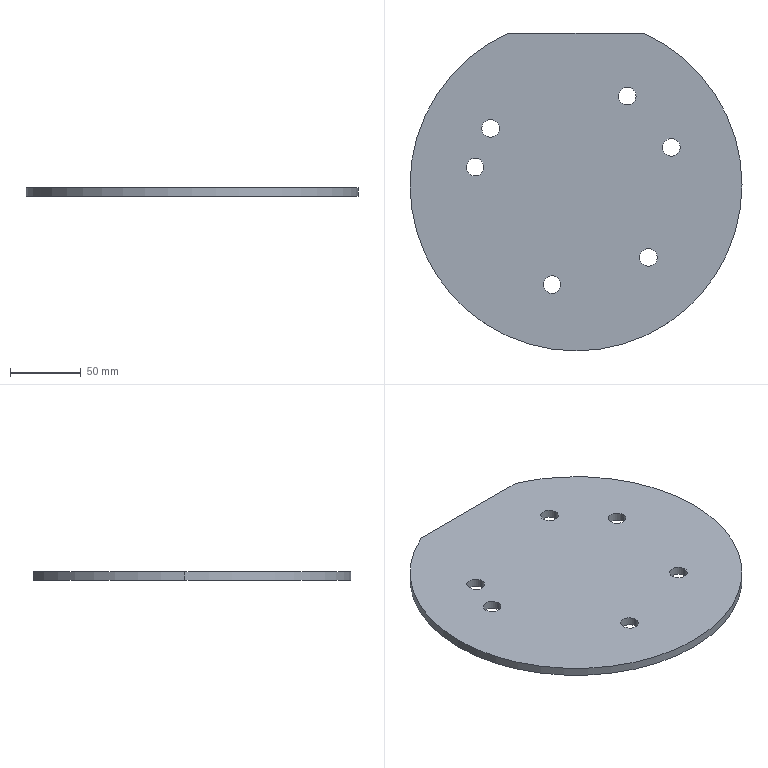Part | SolidWorks | features FlatPattern 1, SMBaseFlange 1, SheetMetal 1 | 1 solid | 18 faces | box 235 x 225 x 6 mm | volume 251996 mm3 | cylinder 15 | plane 3 | commonest cylinder face diameters 12.5 x12 235 x3
STEP:
#1=CARTESIAN_POINT('',(-77.649,12.589,6.));
#2=VERTEX_POINT('',#1);
#3=CARTESIAN_POINT('',(-65.149,12.589,6.));
#4=VERTEX_POINT('',#3);
#5=CARTESIAN_POINT('',(-71.399,12.589,6.));
#6=DIRECTION('',(0.,0.,1.));
#7=DIRECTION('',(1.,0.,0.));
#8=AXIS2_PLACEMENT_3D('',#5,#6,#7);
#9=CIRCLE('',#8,6.25);
#10=EDGE_CURVE('',#2,#4,#9,.T.);
#11=ORIENTED_EDGE('',*,*,#10,.T.);
#12=CARTESIAN_POINT('',(-65.149,12.589,0.));
#13=VERTEX_POINT('',#12);
#14=CARTESIAN_POINT('',(-65.149,12.589,6.));
#15=DIRECTION('',(0.,0.,-1.));
#16=VECTOR('',#15,1000.);
#17=LINE('',#14,#16);
#18=EDGE_CURVE('',#4,#13,#17,.T.);
#19=ORIENTED_EDGE('',*,*,#18,.T.);
#20=CARTESIAN_POINT('',(-77.649,12.589,0.));
#21=VERTEX_POINT('',#20);
#22=CARTESIAN_POINT('',(-71.399,12.589,0.));
#23=DIRECTION('',(0.,0.,1.));
#24=DIRECTION('',(1.,0.,0.));
#25=AXIS2_PLACEMENT_3D('',#22,#23,#24);
#26=CIRCLE('',#25,6.25);
#27=EDGE_CURVE('',#21,#13,#26,.T.);
#28=ORIENTED_EDGE('',*,*,#27,.F.);
#29=CARTESIAN_POINT('',(-77.649,12.589,6.));
#30=DIRECTION('',(0.,0.,-1.));
#31=VECTOR('',#30,1000.);
#32=LINE('',#29,#31);
#33=EDGE_CURVE('',#2,#21,#32,.T.);
#34=ORIENTED_EDGE('',*,*,#33,.F.);
#35=EDGE_LOOP('',(#11,#19,#28,#34));
#36=FACE_OUTER_BOUND('',#35,.T.);
#37=CARTESIAN_POINT('',(-71.399,12.589,6.));
#38=DIRECTION('',(0.,0.,-1.));
#39=DIRECTION('',(-1.,0.,0.));
#40=AXIS2_PLACEMENT_3D('',#37,#38,#39);
#41=CYLINDRICAL_SURFACE('',#40,6.25);
#42=ADVANCED_FACE('',(#36),#41,.F.);
#43=CARTESIAN_POINT('',(-66.707,40.015,6.));
#44=VERTEX_POINT('',#43);
#45=CARTESIAN_POINT('',(-54.207,40.015,6.));
#46=VERTEX_POINT('',#45);
#47=CARTESIAN_POINT('',(-60.457,40.015,6.));
#48=DIRECTION('',(0.,0.,1.));
#49=DIRECTION('',(1.,0.,0.));
#50=AXIS2_PLACEMENT_3D('',#47,#48,#49);
#51=CIRCLE('',#50,6.25);
#52=EDGE_CURVE('',#44,#46,#51,.T.);
#53=ORIENTED_EDGE('',*,*,#52,.T.);
#54=CARTESIAN_POINT('',(-54.207,40.015,0.));
#55=VERTEX_POINT('',#54);
#56=CARTESIAN_POINT('',(-54.207,40.015,6.));
#57=DIRECTION('',(0.,0.,-1.));
#58=VECTOR('',#57,1000.);
#59=LINE('',#56,#58);
#60=EDGE_CURVE('',#46,#55,#59,.T.);
#61=ORIENTED_EDGE('',*,*,#60,.T.);
#62=CARTESIAN_POINT('',(-66.707,40.015,0.));
#63=VERTEX_POINT('',#62);
#64=CARTESIAN_POINT('',(-60.457,40.015,0.));
#65=DIRECTION('',(0.,0.,1.));
#66=DIRECTION('',(1.,0.,0.));
#67=AXIS2_PLACEMENT_3D('',#64,#65,#66);
#68=CIRCLE('',#67,6.25);
#69=EDGE_CURVE('',#63,#55,#68,.T.);
#70=ORIENTED_EDGE('',*,*,#69,.F.);
#71=CARTESIAN_POINT('',(-66.707,40.015,6.));
#72=DIRECTION('',(0.,0.,-1.));
#73=VECTOR('',#72,1000.);
#74=LINE('',#71,#73);
#75=EDGE_CURVE('',#44,#63,#74,.T.);
#76=ORIENTED_EDGE('',*,*,#75,.F.);
#77=EDGE_LOOP('',(#53,#61,#70,#76));
#78=FACE_OUTER_BOUND('',#77,.T.);
#79=CARTESIAN_POINT('',(-60.457,40.015,6.));
#80=DIRECTION('',(0.,0.,-1.));
#81=DIRECTION('',(-1.,0.,0.));
#82=AXIS2_PLACEMENT_3D('',#79,#80,#81);
#83=CYLINDRICAL_SURFACE('',#82,6.25);
#84=ADVANCED_FACE('',(#78),#83,.F.);
#85=CARTESIAN_POINT('',(30.,62.787,6.));
#86=VERTEX_POINT('',#85);
#87=CARTESIAN_POINT('',(42.5,62.787,6.));
#88=VERTEX_POINT('',#87);
#89=CARTESIAN_POINT('',(36.25,62.787,6.));
#90=DIRECTION('',(0.,0.,1.));
#91=DIRECTION('',(1.,0.,0.));
#92=AXIS2_PLACEMENT_3D('',#89,#90,#91);
#93=CIRCLE('',#92,6.25);
#94=EDGE_CURVE('',#86,#88,#93,.T.);
#95=ORIENTED_EDGE('',*,*,#94,.T.);
#96=CARTESIAN_POINT('',(42.5,62.787,0.));
#97=VERTEX_POINT('',#96);
#98=CARTESIAN_POINT('',(42.5,62.787,6.));
#99=DIRECTION('',(0.,0.,-1.));
#100=VECTOR('',#99,1000.);
#101=LINE('',#98,#100);
#102=EDGE_CURVE('',#88,#97,#101,.T.);
#103=ORIENTED_EDGE('',*,*,#102,.T.);
#104=CARTESIAN_POINT('',(30.,62.787,0.));
#105=VERTEX_POINT('',#104);
#106=CARTESIAN_POINT('',(36.25,62.787,0.));
#107=DIRECTION('',(0.,0.,1.));
#108=DIRECTION('',(1.,0.,0.));
#109=AXIS2_PLACEMENT_3D('',#106,#107,#108);
#110=CIRCLE('',#109,6.25);
#111=EDGE_CURVE('',#105,#97,#110,.T.);
#112=ORIENTED_EDGE('',*,*,#111,.F.);
#113=CARTESIAN_POINT('',(30.,62.787,6.));
#114=DIRECTION('',(0.,0.,-1.));
#115=VECTOR('',#114,1000.);
#116=LINE('',#113,#115);
#117=EDGE_CURVE('',#86,#105,#116,.T.);
#118=ORIENTED_EDGE('',*,*,#117,.F.);
#119=EDGE_LOOP('',(#95,#103,#112,#118));
#120=FACE_OUTER_BOUND('',#119,.T.);
#121=CARTESIAN_POINT('',(36.25,62.787,6.));
#122=DIRECTION('',(0.,0.,-1.));
#123=DIRECTION('',(-1.,0.,0.));
#124=AXIS2_PLACEMENT_3D('',#121,#122,#123);
#125=CYLINDRICAL_SURFACE('',#124,6.25);
#126=ADVANCED_FACE('',(#120),#125,.F.);
#127=CARTESIAN_POINT('',(61.205,26.571,6.));
#128=VERTEX_POINT('',#127);
#129=CARTESIAN_POINT('',(73.705,26.571,6.));
#130=VERTEX_POINT('',#129);
#131=CARTESIAN_POINT('',(67.455,26.571,6.));
#132=DIRECTION('',(0.,0.,1.));
#133=DIRECTION('',(1.,0.,0.));
#134=AXIS2_PLACEMENT_3D('',#131,#132,#133);
#135=CIRCLE('',#134,6.25);
#136=EDGE_CURVE('',#128,#130,#135,.T.);
#137=ORIENTED_EDGE('',*,*,#136,.T.);
#138=CARTESIAN_POINT('',(73.705,26.571,0.));
#139=VERTEX_POINT('',#138);
#140=CARTESIAN_POINT('',(73.705,26.571,6.));
#141=DIRECTION('',(0.,0.,-1.));
#142=VECTOR('',#141,1000.);
#143=LINE('',#140,#142);
#144=EDGE_CURVE('',#130,#139,#143,.T.);
#145=ORIENTED_EDGE('',*,*,#144,.T.);
#146=CARTESIAN_POINT('',(61.205,26.571,0.));
#147=VERTEX_POINT('',#146);
#148=CARTESIAN_POINT('',(67.455,26.571,0.));
#149=DIRECTION('',(0.,0.,1.));
#150=DIRECTION('',(1.,0.,0.));
#151=AXIS2_PLACEMENT_3D('',#148,#149,#150);
#152=CIRCLE('',#151,6.25);
#153=EDGE_CURVE('',#147,#139,#152,.T.);
#154=ORIENTED_EDGE('',*,*,#153,.F.);
#155=CARTESIAN_POINT('',(61.205,26.571,6.));
#156=DIRECTION('',(0.,0.,-1.));
#157=VECTOR('',#156,1000.);
#158=LINE('',#155,#157);
#159=EDGE_CURVE('',#128,#147,#158,.T.);
#160=ORIENTED_EDGE('',*,*,#159,.F.);
#161=EDGE_LOOP('',(#137,#145,#154,#160));
#162=FACE_OUTER_BOUND('',#161,.T.);
#163=CARTESIAN_POINT('',(67.455,26.571,6.));
#164=DIRECTION('',(0.,0.,-1.));
#165=DIRECTION('',(-1.,0.,0.));
#166=AXIS2_PLACEMENT_3D('',#163,#164,#165);
#167=CYLINDRICAL_SURFACE('',#166,6.25);
#168=ADVANCED_FACE('',(#162),#167,.F.);
#169=CARTESIAN_POINT('',(45.015,-51.265,6.));
#170=VERTEX_POINT('',#169);
#171=CARTESIAN_POINT('',(57.515,-51.265,6.));
#172=VERTEX_POINT('',#171);
#173=CARTESIAN_POINT('',(51.265,-51.265,6.));
#174=DIRECTION('',(0.,0.,1.));
#175=DIRECTION('',(1.,0.,0.));
#176=AXIS2_PLACEMENT_3D('',#173,#174,#175);
#177=CIRCLE('',#176,6.25);
#178=EDGE_CURVE('',#170,#172,#177,.T.);
#179=ORIENTED_EDGE('',*,*,#178,.T.);
#180=CARTESIAN_POINT('',(57.515,-51.265,0.));
#181=VERTEX_POINT('',#180);
#182=CARTESIAN_POINT('',(57.515,-51.265,6.));
#183=DIRECTION('',(0.,0.,-1.));
#184=VECTOR('',#183,1000.);
#185=LINE('',#182,#184);
#186=EDGE_CURVE('',#172,#181,#185,.T.);
#187=ORIENTED_EDGE('',*,*,#186,.T.);
#188=CARTESIAN_POINT('',(45.015,-51.265,0.));
#189=VERTEX_POINT('',#188);
#190=CARTESIAN_POINT('',(51.265,-51.265,0.));
#191=DIRECTION('',(0.,0.,1.));
#192=DIRECTION('',(1.,0.,0.));
#193=AXIS2_PLACEMENT_3D('',#190,#191,#192);
#194=CIRCLE('',#193,6.25);
#195=EDGE_CURVE('',#189,#181,#194,.T.);
#196=ORIENTED_EDGE('',*,*,#195,.F.);
#197=CARTESIAN_POINT('',(45.015,-51.265,6.));
#198=DIRECTION('',(0.,0.,-1.));
#199=VECTOR('',#198,1000.);
#200=LINE('',#197,#199);
#201=EDGE_CURVE('',#170,#189,#200,.T.);
#202=ORIENTED_EDGE('',*,*,#201,.F.);
#203=EDGE_LOOP('',(#179,#187,#196,#202));
#204=FACE_OUTER_BOUND('',#203,.T.);
#205=CARTESIAN_POINT('',(51.265,-51.265,6.));
#206=DIRECTION('',(0.,0.,-1.));
#207=DIRECTION('',(-1.,0.,0.));
#208=AXIS2_PLACEMENT_3D('',#205,#206,#207);
#209=CYLINDRICAL_SURFACE('',#208,6.25);
#210=ADVANCED_FACE('',(#204),#209,.F.);
#211=CARTESIAN_POINT('',(-23.175,-70.497,6.));
#212=VERTEX_POINT('',#211);
#213=CARTESIAN_POINT('',(-10.675,-70.497,6.));
#214=VERTEX_POINT('',#213);
#215=CARTESIAN_POINT('',(-16.925,-70.497,6.));
#216=DIRECTION('',(0.,0.,1.));
#217=DIRECTION('',(1.,0.,0.));
#218=AXIS2_PLACEMENT_3D('',#215,#216,#217);
#219=CIRCLE('',#218,6.25);
#220=EDGE_CURVE('',#212,#214,#219,.T.);
#221=ORIENTED_EDGE('',*,*,#220,.T.);
#222=CARTESIAN_POINT('',(-10.675,-70.497,0.));
#223=VERTEX_POINT('',#222);
#224=CARTESIAN_POINT('',(-10.675,-70.497,6.));
#225=DIRECTION('',(0.,0.,-1.));
#226=VECTOR('',#225,1000.);
#227=LINE('',#224,#226);
#228=EDGE_CURVE('',#214,#223,#227,.T.);
#229=ORIENTED_EDGE('',*,*,#228,.T.);
#230=CARTESIAN_POINT('',(-23.175,-70.497,0.));
#231=VERTEX_POINT('',#230);
#232=CARTESIAN_POINT('',(-16.925,-70.497,0.));
#233=DIRECTION('',(0.,0.,1.));
#234=DIRECTION('',(1.,0.,0.));
#235=AXIS2_PLACEMENT_3D('',#232,#233,#234);
#236=CIRCLE('',#235,6.25);
#237=EDGE_CURVE('',#231,#223,#236,.T.);
#238=ORIENTED_EDGE('',*,*,#237,.F.);
#239=CARTESIAN_POINT('',(-23.175,-70.497,6.));
#240=DIRECTION('',(0.,0.,-1.));
#241=VECTOR('',#240,1000.);
#242=LINE('',#239,#241);
#243=EDGE_CURVE('',#212,#231,#242,.T.);
#244=ORIENTED_EDGE('',*,*,#243,.F.);
#245=EDGE_LOOP('',(#221,#229,#238,#244));
#246=FACE_OUTER_BOUND('',#245,.T.);
#247=CARTESIAN_POINT('',(-16.925,-70.497,6.));
#248=DIRECTION('',(0.,0.,-1.));
#249=DIRECTION('',(-1.,0.,0.));
#250=AXIS2_PLACEMENT_3D('',#247,#248,#249);
#251=CYLINDRICAL_SURFACE('',#250,6.25);
#252=ADVANCED_FACE('',(#246),#251,.F.);
#253=CARTESIAN_POINT('',(117.5,0.,6.));
#254=VERTEX_POINT('',#253);
#255=CARTESIAN_POINT('',(47.434,107.5,6.));
#256=VERTEX_POINT('',#255);
#257=CARTESIAN_POINT('',(0.,0.,6.));
#258=DIRECTION('',(0.,0.,1.));
#259=DIRECTION('',(1.,0.,0.));
#260=AXIS2_PLACEMENT_3D('',#257,#258,#259);
#261=CIRCLE('',#260,117.5);
#262=EDGE_CURVE('',#254,#256,#261,.T.);
#263=ORIENTED_EDGE('',*,*,#262,.F.);
#264=CARTESIAN_POINT('',(117.5,0.,0.));
#265=VERTEX_POINT('',#264);
#266=CARTESIAN_POINT('',(117.5,0.,6.));
#267=DIRECTION('',(0.,0.,-1.));
#268=VECTOR('',#267,1000.);
#269=LINE('',#266,#268);
#270=EDGE_CURVE('',#254,#265,#269,.T.);
#271=ORIENTED_EDGE('',*,*,#270,.T.);
#272=CARTESIAN_POINT('',(47.434,107.5,0.));
#273=VERTEX_POINT('',#272);
#274=CARTESIAN_POINT('',(0.,0.,0.));
#275=DIRECTION('',(0.,0.,1.));
#276=DIRECTION('',(1.,0.,0.));
#277=AXIS2_PLACEMENT_3D('',#274,#275,#276);
#278=CIRCLE('',#277,117.5);
#279=EDGE_CURVE('',#265,#273,#278,.T.);
#280=ORIENTED_EDGE('',*,*,#279,.T.);
#281=CARTESIAN_POINT('',(47.434,107.5,6.));
#282=DIRECTION('',(0.,0.,-1.));
#283=VECTOR('',#282,1000.);
#284=LINE('',#281,#283);
#285=EDGE_CURVE('',#256,#273,#284,.T.);
#286=ORIENTED_EDGE('',*,*,#285,.F.);
#287=EDGE_LOOP('',(#263,#271,#280,#286));
#288=FACE_OUTER_BOUND('',#287,.T.);
#289=CARTESIAN_POINT('',(0.,0.,6.));
#290=DIRECTION('',(0.,0.,-1.));
#291=DIRECTION('',(-1.,0.,0.));
#292=AXIS2_PLACEMENT_3D('',#289,#290,#291);
#293=CYLINDRICAL_SURFACE('',#292,117.5);
#294=ADVANCED_FACE('',(#288),#293,.T.);
#295=ORIENTED_EDGE('',*,*,#270,.F.);
#296=CARTESIAN_POINT('',(-117.5,0.,6.));
#297=VERTEX_POINT('',#296);
#298=CARTESIAN_POINT('',(0.,0.,6.));
#299=DIRECTION('',(0.,0.,1.));
#300=DIRECTION('',(1.,0.,0.));
#301=AXIS2_PLACEMENT_3D('',#298,#299,#300);
#302=CIRCLE('',#301,117.5);
#303=EDGE_CURVE('',#297,#254,#302,.T.);
#304=ORIENTED_EDGE('',*,*,#303,.F.);
#305=CARTESIAN_POINT('',(-117.5,0.,0.));
#306=VERTEX_POINT('',#305);
#307=CARTESIAN_POINT('',(-117.5,0.,6.));
#308=DIRECTION('',(0.,0.,-1.));
#309=VECTOR('',#308,1000.);
#310=LINE('',#307,#309);
#311=EDGE_CURVE('',#297,#306,#310,.T.);
#312=ORIENTED_EDGE('',*,*,#311,.T.);
#313=CARTESIAN_POINT('',(0.,0.,0.));
#314=DIRECTION('',(0.,0.,1.));
#315=DIRECTION('',(1.,0.,0.));
#316=AXIS2_PLACEMENT_3D('',#313,#314,#315);
#317=CIRCLE('',#316,117.5);
#318=EDGE_CURVE('',#306,#265,#317,.T.);
#319=ORIENTED_EDGE('',*,*,#318,.T.);
#320=EDGE_LOOP('',(#295,#304,#312,#319));
#321=FACE_OUTER_BOUND('',#320,.T.);
#322=CARTESIAN_POINT('',(0.,0.,6.));
#323=DIRECTION('',(0.,0.,-1.));
#324=DIRECTION('',(-1.,0.,0.));
#325=AXIS2_PLACEMENT_3D('',#322,#323,#324);
#326=CYLINDRICAL_SURFACE('',#325,117.5);
#327=ADVANCED_FACE('',(#321),#326,.T.);
#328=ORIENTED_EDGE('',*,*,#52,.F.);
#329=CARTESIAN_POINT('',(-60.457,40.015,6.));
#330=DIRECTION('',(0.,0.,1.));
#331=DIRECTION('',(1.,0.,0.));
#332=AXIS2_PLACEMENT_3D('',#329,#330,#331);
#333=CIRCLE('',#332,6.25);
#334=EDGE_CURVE('',#46,#44,#333,.T.);
#335=ORIENTED_EDGE('',*,*,#334,.F.);
#336=EDGE_LOOP('',(#328,#335));
#337=FACE_BOUND('',#336,.T.);
#338=ORIENTED_EDGE('',*,*,#136,.F.);
#339=CARTESIAN_POINT('',(67.455,26.571,6.));
#340=DIRECTION('',(0.,0.,1.));
#341=DIRECTION('',(1.,0.,0.));
#342=AXIS2_PLACEMENT_3D('',#339,#340,#341);
#343=CIRCLE('',#342,6.25);
#344=EDGE_CURVE('',#130,#128,#343,.T.);
#345=ORIENTED_EDGE('',*,*,#344,.F.);
#346=EDGE_LOOP('',(#338,#345));
#347=FACE_BOUND('',#346,.T.);
#348=ORIENTED_EDGE('',*,*,#220,.F.);
#349=CARTESIAN_POINT('',(-16.925,-70.497,6.));
#350=DIRECTION('',(0.,0.,1.));
#351=DIRECTION('',(1.,0.,0.));
#352=AXIS2_PLACEMENT_3D('',#349,#350,#351);
#353=CIRCLE('',#352,6.25);
#354=EDGE_CURVE('',#214,#212,#353,.T.);
#355=ORIENTED_EDGE('',*,*,#354,.F.);
#356=EDGE_LOOP('',(#348,#355));
#357=FACE_BOUND('',#356,.T.);
#358=CARTESIAN_POINT('',(-47.434,107.5,6.));
#359=VERTEX_POINT('',#358);
#360=CARTESIAN_POINT('',(0.,0.,6.));
#361=DIRECTION('',(0.,0.,1.));
#362=DIRECTION('',(1.,0.,0.));
#363=AXIS2_PLACEMENT_3D('',#360,#361,#362);
#364=CIRCLE('',#363,117.5);
#365=EDGE_CURVE('',#359,#297,#364,.T.);
#366=ORIENTED_EDGE('',*,*,#365,.T.);
#367=ORIENTED_EDGE('',*,*,#303,.T.);
#368=ORIENTED_EDGE('',*,*,#262,.T.);
#369=CARTESIAN_POINT('',(47.434,107.5,6.));
#370=DIRECTION('',(-1.,0.,0.));
#371=VECTOR('',#370,1000.);
#372=LINE('',#369,#371);
#373=EDGE_CURVE('',#256,#359,#372,.T.);
#374=ORIENTED_EDGE('',*,*,#373,.T.);
#375=EDGE_LOOP('',(#366,#367,#368,#374));
#376=FACE_OUTER_BOUND('',#375,.T.);
#377=ORIENTED_EDGE('',*,*,#178,.F.);
#378=CARTESIAN_POINT('',(51.265,-51.265,6.));
#379=DIRECTION('',(0.,0.,1.));
#380=DIRECTION('',(1.,0.,0.));
#381=AXIS2_PLACEMENT_3D('',#378,#379,#380);
#382=CIRCLE('',#381,6.25);
#383=EDGE_CURVE('',#172,#170,#382,.T.);
#384=ORIENTED_EDGE('',*,*,#383,.F.);
#385=EDGE_LOOP('',(#377,#384));
#386=FACE_BOUND('',#385,.T.);
#387=ORIENTED_EDGE('',*,*,#94,.F.);
#388=CARTESIAN_POINT('',(36.25,62.787,6.));
#389=DIRECTION('',(0.,0.,1.));
#390=DIRECTION('',(1.,0.,0.));
#391=AXIS2_PLACEMENT_3D('',#388,#389,#390);
#392=CIRCLE('',#391,6.25);
#393=EDGE_CURVE('',#88,#86,#392,.T.);
#394=ORIENTED_EDGE('',*,*,#393,.F.);
#395=EDGE_LOOP('',(#387,#394));
#396=FACE_BOUND('',#395,.T.);
#397=ORIENTED_EDGE('',*,*,#10,.F.);
#398=CARTESIAN_POINT('',(-71.399,12.589,6.));
#399=DIRECTION('',(0.,0.,1.));
#400=DIRECTION('',(1.,0.,0.));
#401=AXIS2_PLACEMENT_3D('',#398,#399,#400);
#402=CIRCLE('',#401,6.25);
#403=EDGE_CURVE('',#4,#2,#402,.T.);
#404=ORIENTED_EDGE('',*,*,#403,.F.);
#405=EDGE_LOOP('',(#397,#404));
#406=FACE_BOUND('',#405,.T.);
#407=CARTESIAN_POINT('',(0.,0.,6.));
#408=DIRECTION('',(0.,0.,1.));
#409=DIRECTION('',(1.,0.,0.));
#410=AXIS2_PLACEMENT_3D('',#407,#408,#409);
#411=PLANE('',#410);
#412=ADVANCED_FACE('',(#337,#347,#357,#376,#386,#396,#406),#411,.T.);
#413=CARTESIAN_POINT('',(-47.434,107.5,0.));
#414=VERTEX_POINT('',#413);
#415=CARTESIAN_POINT('',(0.,0.,0.));
#416=DIRECTION('',(0.,0.,1.));
#417=DIRECTION('',(1.,0.,0.));
#418=AXIS2_PLACEMENT_3D('',#415,#416,#417);
#419=CIRCLE('',#418,117.5);
#420=EDGE_CURVE('',#414,#306,#419,.T.);
#421=ORIENTED_EDGE('',*,*,#420,.F.);
#422=CARTESIAN_POINT('',(47.434,107.5,0.));
#423=DIRECTION('',(-1.,0.,0.));
#424=VECTOR('',#423,1000.);
#425=LINE('',#422,#424);
#426=EDGE_CURVE('',#273,#414,#425,.T.);
#427=ORIENTED_EDGE('',*,*,#426,.F.);
#428=ORIENTED_EDGE('',*,*,#279,.F.);
#429=ORIENTED_EDGE('',*,*,#318,.F.);
#430=EDGE_LOOP('',(#421,#427,#428,#429));
#431=FACE_OUTER_BOUND('',#430,.T.);
#432=ORIENTED_EDGE('',*,*,#237,.T.);
#433=CARTESIAN_POINT('',(-16.925,-70.497,0.));
#434=DIRECTION('',(0.,0.,1.));
#435=DIRECTION('',(1.,0.,0.));
#436=AXIS2_PLACEMENT_3D('',#433,#434,#435);
#437=CIRCLE('',#436,6.25);
#438=EDGE_CURVE('',#223,#231,#437,.T.);
#439=ORIENTED_EDGE('',*,*,#438,.T.);
#440=EDGE_LOOP('',(#432,#439));
#441=FACE_BOUND('',#440,.T.);
#442=ORIENTED_EDGE('',*,*,#195,.T.);
#443=CARTESIAN_POINT('',(51.265,-51.265,0.));
#444=DIRECTION('',(0.,0.,1.));
#445=DIRECTION('',(1.,0.,0.));
#446=AXIS2_PLACEMENT_3D('',#443,#444,#445);
#447=CIRCLE('',#446,6.25);
#448=EDGE_CURVE('',#181,#189,#447,.T.);
#449=ORIENTED_EDGE('',*,*,#448,.T.);
#450=EDGE_LOOP('',(#442,#449));
#451=FACE_BOUND('',#450,.T.);
#452=ORIENTED_EDGE('',*,*,#153,.T.);
#453=CARTESIAN_POINT('',(67.455,26.571,0.));
#454=DIRECTION('',(0.,0.,1.));
#455=DIRECTION('',(1.,0.,0.));
#456=AXIS2_PLACEMENT_3D('',#453,#454,#455);
#457=CIRCLE('',#456,6.25);
#458=EDGE_CURVE('',#139,#147,#457,.T.);
#459=ORIENTED_EDGE('',*,*,#458,.T.);
#460=EDGE_LOOP('',(#452,#459));
#461=FACE_BOUND('',#460,.T.);
#462=ORIENTED_EDGE('',*,*,#111,.T.);
#463=CARTESIAN_POINT('',(36.25,62.787,0.));
#464=DIRECTION('',(0.,0.,1.));
#465=DIRECTION('',(1.,0.,0.));
#466=AXIS2_PLACEMENT_3D('',#463,#464,#465);
#467=CIRCLE('',#466,6.25);
#468=EDGE_CURVE('',#97,#105,#467,.T.);
#469=ORIENTED_EDGE('',*,*,#468,.T.);
#470=EDGE_LOOP('',(#462,#469));
#471=FACE_BOUND('',#470,.T.);
#472=ORIENTED_EDGE('',*,*,#69,.T.);
#473=CARTESIAN_POINT('',(-60.457,40.015,0.));
#474=DIRECTION('',(0.,0.,1.));
#475=DIRECTION('',(1.,0.,0.));
#476=AXIS2_PLACEMENT_3D('',#473,#474,#475);
#477=CIRCLE('',#476,6.25);
#478=EDGE_CURVE('',#55,#63,#477,.T.);
#479=ORIENTED_EDGE('',*,*,#478,.T.);
#480=EDGE_LOOP('',(#472,#479));
#481=FACE_BOUND('',#480,.T.);
#482=ORIENTED_EDGE('',*,*,#27,.T.);
#483=CARTESIAN_POINT('',(-71.399,12.589,0.));
#484=DIRECTION('',(0.,0.,1.));
#485=DIRECTION('',(1.,0.,0.));
#486=AXIS2_PLACEMENT_3D('',#483,#484,#485);
#487=CIRCLE('',#486,6.25);
#488=EDGE_CURVE('',#13,#21,#487,.T.);
#489=ORIENTED_EDGE('',*,*,#488,.T.);
#490=EDGE_LOOP('',(#482,#489));
#491=FACE_BOUND('',#490,.T.);
#492=CARTESIAN_POINT('',(0.,0.,0.));
#493=DIRECTION('',(0.,0.,1.));
#494=DIRECTION('',(1.,0.,0.));
#495=AXIS2_PLACEMENT_3D('',#492,#493,#494);
#496=PLANE('',#495);
#497=ADVANCED_FACE('',(#431,#441,#451,#461,#471,#481,#491),#496,.F.);
#498=ORIENTED_EDGE('',*,*,#311,.F.);
#499=ORIENTED_EDGE('',*,*,#365,.F.);
#500=CARTESIAN_POINT('',(-47.434,107.5,6.));
#501=DIRECTION('',(0.,0.,-1.));
#502=VECTOR('',#501,1000.);
#503=LINE('',#500,#502);
#504=EDGE_CURVE('',#359,#414,#503,.T.);
#505=ORIENTED_EDGE('',*,*,#504,.T.);
#506=ORIENTED_EDGE('',*,*,#420,.T.);
#507=EDGE_LOOP('',(#498,#499,#505,#506));
#508=FACE_OUTER_BOUND('',#507,.T.);
#509=CARTESIAN_POINT('',(0.,0.,6.));
#510=DIRECTION('',(0.,0.,-1.));
#511=DIRECTION('',(-1.,0.,0.));
#512=AXIS2_PLACEMENT_3D('',#509,#510,#511);
#513=CYLINDRICAL_SURFACE('',#512,117.5);
#514=ADVANCED_FACE('',(#508),#513,.T.);
#515=ORIENTED_EDGE('',*,*,#426,.T.);
#516=ORIENTED_EDGE('',*,*,#504,.F.);
#517=ORIENTED_EDGE('',*,*,#373,.F.);
#518=ORIENTED_EDGE('',*,*,#285,.T.);
#519=EDGE_LOOP('',(#515,#516,#517,#518));
#520=FACE_OUTER_BOUND('',#519,.T.);
#521=CARTESIAN_POINT('',(47.434,107.5,6.));
#522=DIRECTION('',(0.,-1.,0.));
#523=DIRECTION('',(0.,0.,-1.));
#524=AXIS2_PLACEMENT_3D('',#521,#522,#523);
#525=PLANE('',#524);
#526=ADVANCED_FACE('',(#520),#525,.F.);
#527=ORIENTED_EDGE('',*,*,#228,.F.);
#528=ORIENTED_EDGE('',*,*,#354,.T.);
#529=ORIENTED_EDGE('',*,*,#243,.T.);
#530=ORIENTED_EDGE('',*,*,#438,.F.);
#531=EDGE_LOOP('',(#527,#528,#529,#530));
#532=FACE_OUTER_BOUND('',#531,.T.);
#533=CARTESIAN_POINT('',(-16.925,-70.497,6.));
#534=DIRECTION('',(0.,0.,-1.));
#535=DIRECTION('',(-1.,0.,0.));
#536=AXIS2_PLACEMENT_3D('',#533,#534,#535);
#537=CYLINDRICAL_SURFACE('',#536,6.25);
#538=ADVANCED_FACE('',(#532),#537,.F.);
#539=ORIENTED_EDGE('',*,*,#186,.F.);
#540=ORIENTED_EDGE('',*,*,#383,.T.);
#541=ORIENTED_EDGE('',*,*,#201,.T.);
#542=ORIENTED_EDGE('',*,*,#448,.F.);
#543=EDGE_LOOP('',(#539,#540,#541,#542));
#544=FACE_OUTER_BOUND('',#543,.T.);
#545=CARTESIAN_POINT('',(51.265,-51.265,6.));
#546=DIRECTION('',(0.,0.,-1.));
#547=DIRECTION('',(-1.,0.,0.));
#548=AXIS2_PLACEMENT_3D('',#545,#546,#547);
#549=CYLINDRICAL_SURFACE('',#548,6.25);
#550=ADVANCED_FACE('',(#544),#549,.F.);
#551=ORIENTED_EDGE('',*,*,#144,.F.);
#552=ORIENTED_EDGE('',*,*,#344,.T.);
#553=ORIENTED_EDGE('',*,*,#159,.T.);
#554=ORIENTED_EDGE('',*,*,#458,.F.);
#555=EDGE_LOOP('',(#551,#552,#553,#554));
#556=FACE_OUTER_BOUND('',#555,.T.);
#557=CARTESIAN_POINT('',(67.455,26.571,6.));
#558=DIRECTION('',(0.,0.,-1.));
#559=DIRECTION('',(-1.,0.,0.));
#560=AXIS2_PLACEMENT_3D('',#557,#558,#559);
#561=CYLINDRICAL_SURFACE('',#560,6.25);
#562=ADVANCED_FACE('',(#556),#561,.F.);
#563=ORIENTED_EDGE('',*,*,#102,.F.);
#564=ORIENTED_EDGE('',*,*,#393,.T.);
#565=ORIENTED_EDGE('',*,*,#117,.T.);
#566=ORIENTED_EDGE('',*,*,#468,.F.);
#567=EDGE_LOOP('',(#563,#564,#565,#566));
#568=FACE_OUTER_BOUND('',#567,.T.);
#569=CARTESIAN_POINT('',(36.25,62.787,6.));
#570=DIRECTION('',(0.,0.,-1.));
#571=DIRECTION('',(-1.,0.,0.));
#572=AXIS2_PLACEMENT_3D('',#569,#570,#571);
#573=CYLINDRICAL_SURFACE('',#572,6.25);
#574=ADVANCED_FACE('',(#568),#573,.F.);
#575=ORIENTED_EDGE('',*,*,#60,.F.);
#576=ORIENTED_EDGE('',*,*,#334,.T.);
#577=ORIENTED_EDGE('',*,*,#75,.T.);
#578=ORIENTED_EDGE('',*,*,#478,.F.);
#579=EDGE_LOOP('',(#575,#576,#577,#578));
#580=FACE_OUTER_BOUND('',#579,.T.);
#581=CARTESIAN_POINT('',(-60.457,40.015,6.));
#582=DIRECTION('',(0.,0.,-1.));
#583=DIRECTION('',(-1.,0.,0.));
#584=AXIS2_PLACEMENT_3D('',#581,#582,#583);
#585=CYLINDRICAL_SURFACE('',#584,6.25);
#586=ADVANCED_FACE('',(#580),#585,.F.);
#587=ORIENTED_EDGE('',*,*,#18,.F.);
#588=ORIENTED_EDGE('',*,*,#403,.T.);
#589=ORIENTED_EDGE('',*,*,#33,.T.);
#590=ORIENTED_EDGE('',*,*,#488,.F.);
#591=EDGE_LOOP('',(#587,#588,#589,#590));
#592=FACE_OUTER_BOUND('',#591,.T.);
#593=CARTESIAN_POINT('',(-71.399,12.589,6.));
#594=DIRECTION('',(0.,0.,-1.));
#595=DIRECTION('',(-1.,0.,0.));
#596=AXIS2_PLACEMENT_3D('',#593,#594,#595);
#597=CYLINDRICAL_SURFACE('',#596,6.25);
#598=ADVANCED_FACE('',(#592),#597,.F.);
#599=CLOSED_SHELL('',(#42,#84,#126,#168,#210,#252,#294,#327,#412,#497,#514,#526,#538,#550,#562,#574,#586,#598));
#600=MANIFOLD_SOLID_BREP('',#599);
#601=CARTESIAN_POINT('',(0.,0.,0.));
#602=DIRECTION('',(0.,0.,1.));
#603=DIRECTION('',(1.,0.,0.));
#604=AXIS2_PLACEMENT_3D('',#601,#602,#603);
#605=(LENGTH_UNIT()NAMED_UNIT(*)SI_UNIT(.MILLI.,.METRE.));
#606=UNCERTAINTY_MEASURE_WITH_UNIT(LENGTH_MEASURE(0.00001),#605,'','');
#607=(NAMED_UNIT(*)PLANE_ANGLE_UNIT()SI_UNIT($,.RADIAN.));
#608=(NAMED_UNIT(*)SI_UNIT($,.STERADIAN.)SOLID_ANGLE_UNIT());
#609=(GEOMETRIC_REPRESENTATION_CONTEXT(3)GLOBAL_UNCERTAINTY_ASSIGNED_CONTEXT((#606))GLOBAL_UNIT_ASSIGNED_CONTEXT((#605,#607,#608))REPRESENTATION_CONTEXT('',''));
#610=ADVANCED_BREP_SHAPE_REPRESENTATION('',(#600,#604),#609);